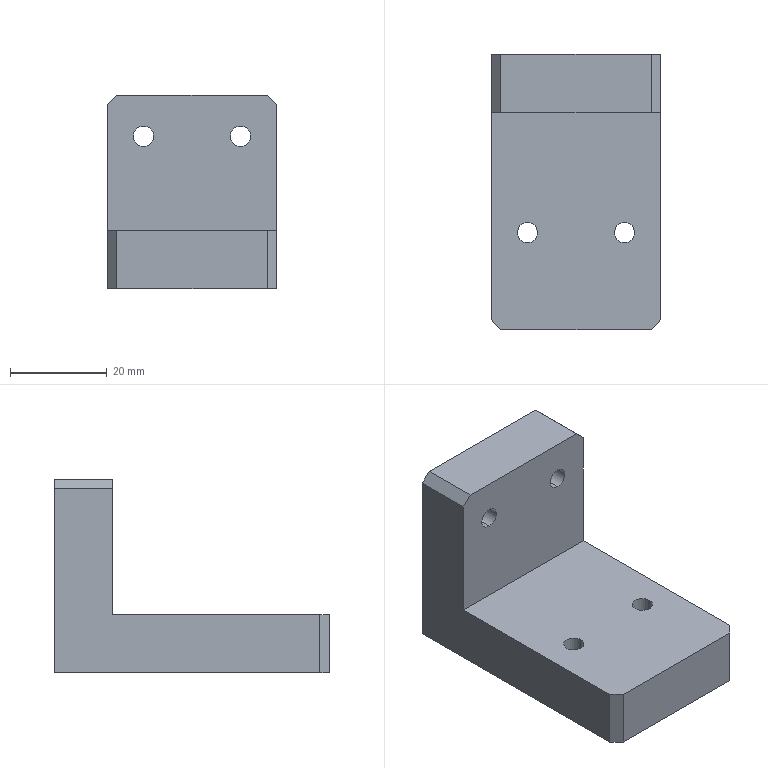Part | SolidWorks | features Chamfer 2, HoleWzd 2, Extrusion 1, ICE 1 | 1 solid | 28 faces | box 35 x 56.7 x 40 mm | volume 34458 mm3 | cylinder 12 | plane 12 | cone 4 | commonest cylinder face diameters 4.2 x12
STEP:
#1=CARTESIAN_POINT('',(-10.,15.95,4.4));
#2=VERTEX_POINT('',#1);
#3=CARTESIAN_POINT('',(-10.,15.95,8.6));
#4=VERTEX_POINT('',#3);
#5=CARTESIAN_POINT('',(-10.,15.95,6.5));
#6=DIRECTION('',(0.,1.,0.));
#7=DIRECTION('',(0.,0.,1.));
#8=AXIS2_PLACEMENT_3D('',#5,#6,#7);
#9=CIRCLE('',#8,2.1);
#10=EDGE_CURVE('',#2,#4,#9,.T.);
#11=ORIENTED_EDGE('',*,*,#10,.F.);
#12=CARTESIAN_POINT('',(-10.,28.35,4.4));
#13=VERTEX_POINT('',#12);
#14=CARTESIAN_POINT('',(-10.,28.35,4.4));
#15=DIRECTION('',(0.,1.,0.));
#16=VECTOR('',#15,1000.);
#17=LINE('',#14,#16);
#18=EDGE_CURVE('',#2,#13,#17,.T.);
#19=ORIENTED_EDGE('',*,*,#18,.T.);
#20=CARTESIAN_POINT('',(-10.,28.35,8.6));
#21=VERTEX_POINT('',#20);
#22=CARTESIAN_POINT('',(-10.,28.35,6.5));
#23=DIRECTION('',(0.,1.,0.));
#24=DIRECTION('',(0.,0.,1.));
#25=AXIS2_PLACEMENT_3D('',#22,#23,#24);
#26=CIRCLE('',#25,2.1);
#27=EDGE_CURVE('',#13,#21,#26,.T.);
#28=ORIENTED_EDGE('',*,*,#27,.T.);
#29=CARTESIAN_POINT('',(-10.,28.35,8.6));
#30=DIRECTION('',(0.,1.,0.));
#31=VECTOR('',#30,1000.);
#32=LINE('',#29,#31);
#33=EDGE_CURVE('',#4,#21,#32,.T.);
#34=ORIENTED_EDGE('',*,*,#33,.F.);
#35=EDGE_LOOP('',(#11,#19,#28,#34));
#36=FACE_OUTER_BOUND('',#35,.T.);
#37=CARTESIAN_POINT('',(-10.,28.35,6.5));
#38=DIRECTION('',(0.,1.,0.));
#39=DIRECTION('',(0.,0.,1.));
#40=AXIS2_PLACEMENT_3D('',#37,#38,#39);
#41=CYLINDRICAL_SURFACE('',#40,2.1);
#42=ADVANCED_FACE('',(#36),#41,.F.);
#43=CARTESIAN_POINT('',(-10.,14.688,6.5));
#44=VERTEX_POINT('',#43);
#45=CARTESIAN_POINT('',(-10.,15.95,8.6));
#46=DIRECTION('',(0.,0.515,0.8572));
#47=VECTOR('',#46,1000.);
#48=LINE('',#45,#47);
#49=EDGE_CURVE('',#44,#4,#48,.T.);
#50=ORIENTED_EDGE('',*,*,#49,.F.);
#51=CARTESIAN_POINT('',(-10.,15.95,4.4));
#52=DIRECTION('',(0.,0.515,-0.8572));
#53=VECTOR('',#52,1000.);
#54=LINE('',#51,#53);
#55=EDGE_CURVE('',#44,#2,#54,.T.);
#56=ORIENTED_EDGE('',*,*,#55,.T.);
#57=ORIENTED_EDGE('',*,*,#10,.T.);
#58=EDGE_LOOP('',(#50,#56,#57));
#59=FACE_OUTER_BOUND('',#58,.T.);
#60=CARTESIAN_POINT('',(-10.,15.95,6.5));
#61=DIRECTION('',(0.,1.,0.));
#62=DIRECTION('',(0.,0.,1.));
#63=AXIS2_PLACEMENT_3D('',#60,#61,#62);
#64=CONICAL_SURFACE('',#63,2.1,1.03);
#65=ADVANCED_FACE('',(#59),#64,.F.);
#66=CARTESIAN_POINT('',(10.,15.95,4.4));
#67=VERTEX_POINT('',#66);
#68=CARTESIAN_POINT('',(10.,15.95,8.6));
#69=VERTEX_POINT('',#68);
#70=CARTESIAN_POINT('',(10.,15.95,6.5));
#71=DIRECTION('',(0.,1.,0.));
#72=DIRECTION('',(0.,0.,1.));
#73=AXIS2_PLACEMENT_3D('',#70,#71,#72);
#74=CIRCLE('',#73,2.1);
#75=EDGE_CURVE('',#67,#69,#74,.T.);
#76=ORIENTED_EDGE('',*,*,#75,.F.);
#77=CARTESIAN_POINT('',(10.,28.35,4.4));
#78=VERTEX_POINT('',#77);
#79=CARTESIAN_POINT('',(10.,28.35,4.4));
#80=DIRECTION('',(0.,1.,0.));
#81=VECTOR('',#80,1000.);
#82=LINE('',#79,#81);
#83=EDGE_CURVE('',#67,#78,#82,.T.);
#84=ORIENTED_EDGE('',*,*,#83,.T.);
#85=CARTESIAN_POINT('',(10.,28.35,8.6));
#86=VERTEX_POINT('',#85);
#87=CARTESIAN_POINT('',(10.,28.35,6.5));
#88=DIRECTION('',(0.,1.,0.));
#89=DIRECTION('',(0.,0.,1.));
#90=AXIS2_PLACEMENT_3D('',#87,#88,#89);
#91=CIRCLE('',#90,2.1);
#92=EDGE_CURVE('',#78,#86,#91,.T.);
#93=ORIENTED_EDGE('',*,*,#92,.T.);
#94=CARTESIAN_POINT('',(10.,28.35,8.6));
#95=DIRECTION('',(0.,1.,0.));
#96=VECTOR('',#95,1000.);
#97=LINE('',#94,#96);
#98=EDGE_CURVE('',#69,#86,#97,.T.);
#99=ORIENTED_EDGE('',*,*,#98,.F.);
#100=EDGE_LOOP('',(#76,#84,#93,#99));
#101=FACE_OUTER_BOUND('',#100,.T.);
#102=CARTESIAN_POINT('',(10.,28.35,6.5));
#103=DIRECTION('',(0.,1.,0.));
#104=DIRECTION('',(0.,0.,1.));
#105=AXIS2_PLACEMENT_3D('',#102,#103,#104);
#106=CYLINDRICAL_SURFACE('',#105,2.1);
#107=ADVANCED_FACE('',(#101),#106,.F.);
#108=CARTESIAN_POINT('',(10.,14.688,6.5));
#109=VERTEX_POINT('',#108);
#110=CARTESIAN_POINT('',(10.,15.95,8.6));
#111=DIRECTION('',(0.,0.515,0.8572));
#112=VECTOR('',#111,1000.);
#113=LINE('',#110,#112);
#114=EDGE_CURVE('',#109,#69,#113,.T.);
#115=ORIENTED_EDGE('',*,*,#114,.F.);
#116=CARTESIAN_POINT('',(10.,15.95,4.4));
#117=DIRECTION('',(0.,0.515,-0.8572));
#118=VECTOR('',#117,1000.);
#119=LINE('',#116,#118);
#120=EDGE_CURVE('',#109,#67,#119,.T.);
#121=ORIENTED_EDGE('',*,*,#120,.T.);
#122=ORIENTED_EDGE('',*,*,#75,.T.);
#123=EDGE_LOOP('',(#115,#121,#122));
#124=FACE_OUTER_BOUND('',#123,.T.);
#125=CARTESIAN_POINT('',(10.,15.95,6.5));
#126=DIRECTION('',(0.,1.,0.));
#127=DIRECTION('',(0.,0.,1.));
#128=AXIS2_PLACEMENT_3D('',#125,#126,#127);
#129=CONICAL_SURFACE('',#128,2.1,1.03);
#130=ADVANCED_FACE('',(#124),#129,.F.);
#131=CARTESIAN_POINT('',(-10.,16.35,33.6));
#132=VERTEX_POINT('',#131);
#133=CARTESIAN_POINT('',(-10.,16.35,29.4));
#134=VERTEX_POINT('',#133);
#135=CARTESIAN_POINT('',(-10.,16.35,31.5));
#136=DIRECTION('',(0.,-1.,0.));
#137=DIRECTION('',(0.,0.,-1.));
#138=AXIS2_PLACEMENT_3D('',#135,#136,#137);
#139=CIRCLE('',#138,2.1);
#140=EDGE_CURVE('',#132,#134,#139,.T.);
#141=ORIENTED_EDGE('',*,*,#140,.T.);
#142=CARTESIAN_POINT('',(-10.,28.35,29.4));
#143=VERTEX_POINT('',#142);
#144=CARTESIAN_POINT('',(-10.,28.35,29.4));
#145=DIRECTION('',(0.,1.,0.));
#146=VECTOR('',#145,1000.);
#147=LINE('',#144,#146);
#148=EDGE_CURVE('',#134,#143,#147,.T.);
#149=ORIENTED_EDGE('',*,*,#148,.T.);
#150=CARTESIAN_POINT('',(-10.,28.35,33.6));
#151=VERTEX_POINT('',#150);
#152=CARTESIAN_POINT('',(-10.,28.35,31.5));
#153=DIRECTION('',(0.,1.,0.));
#154=DIRECTION('',(0.,0.,1.));
#155=AXIS2_PLACEMENT_3D('',#152,#153,#154);
#156=CIRCLE('',#155,2.1);
#157=EDGE_CURVE('',#143,#151,#156,.T.);
#158=ORIENTED_EDGE('',*,*,#157,.T.);
#159=CARTESIAN_POINT('',(-10.,28.35,33.6));
#160=DIRECTION('',(0.,1.,0.));
#161=VECTOR('',#160,1000.);
#162=LINE('',#159,#161);
#163=EDGE_CURVE('',#132,#151,#162,.T.);
#164=ORIENTED_EDGE('',*,*,#163,.F.);
#165=EDGE_LOOP('',(#141,#149,#158,#164));
#166=FACE_OUTER_BOUND('',#165,.T.);
#167=CARTESIAN_POINT('',(-10.,28.35,31.5));
#168=DIRECTION('',(0.,1.,0.));
#169=DIRECTION('',(0.,0.,1.));
#170=AXIS2_PLACEMENT_3D('',#167,#168,#169);
#171=CYLINDRICAL_SURFACE('',#170,2.1);
#172=ADVANCED_FACE('',(#166),#171,.F.);
#173=CARTESIAN_POINT('',(10.,16.35,33.6));
#174=VERTEX_POINT('',#173);
#175=CARTESIAN_POINT('',(10.,16.35,29.4));
#176=VERTEX_POINT('',#175);
#177=CARTESIAN_POINT('',(10.,16.35,31.5));
#178=DIRECTION('',(0.,-1.,0.));
#179=DIRECTION('',(0.,0.,-1.));
#180=AXIS2_PLACEMENT_3D('',#177,#178,#179);
#181=CIRCLE('',#180,2.1);
#182=EDGE_CURVE('',#174,#176,#181,.T.);
#183=ORIENTED_EDGE('',*,*,#182,.T.);
#184=CARTESIAN_POINT('',(10.,28.35,29.4));
#185=VERTEX_POINT('',#184);
#186=CARTESIAN_POINT('',(10.,28.35,29.4));
#187=DIRECTION('',(0.,1.,0.));
#188=VECTOR('',#187,1000.);
#189=LINE('',#186,#188);
#190=EDGE_CURVE('',#176,#185,#189,.T.);
#191=ORIENTED_EDGE('',*,*,#190,.T.);
#192=CARTESIAN_POINT('',(10.,28.35,33.6));
#193=VERTEX_POINT('',#192);
#194=CARTESIAN_POINT('',(10.,28.35,31.5));
#195=DIRECTION('',(0.,1.,0.));
#196=DIRECTION('',(0.,0.,1.));
#197=AXIS2_PLACEMENT_3D('',#194,#195,#196);
#198=CIRCLE('',#197,2.1);
#199=EDGE_CURVE('',#185,#193,#198,.T.);
#200=ORIENTED_EDGE('',*,*,#199,.T.);
#201=CARTESIAN_POINT('',(10.,28.35,33.6));
#202=DIRECTION('',(0.,1.,0.));
#203=VECTOR('',#202,1000.);
#204=LINE('',#201,#203);
#205=EDGE_CURVE('',#174,#193,#204,.T.);
#206=ORIENTED_EDGE('',*,*,#205,.F.);
#207=EDGE_LOOP('',(#183,#191,#200,#206));
#208=FACE_OUTER_BOUND('',#207,.T.);
#209=CARTESIAN_POINT('',(10.,28.35,31.5));
#210=DIRECTION('',(0.,1.,0.));
#211=DIRECTION('',(0.,0.,1.));
#212=AXIS2_PLACEMENT_3D('',#209,#210,#211);
#213=CYLINDRICAL_SURFACE('',#212,2.1);
#214=ADVANCED_FACE('',(#208),#213,.F.);
#215=CARTESIAN_POINT('',(12.1,-8.35,12.));
#216=VERTEX_POINT('',#215);
#217=CARTESIAN_POINT('',(7.9,-8.35,12.));
#218=VERTEX_POINT('',#217);
#219=CARTESIAN_POINT('',(10.,-8.35,12.));
#220=DIRECTION('',(0.,0.,-1.));
#221=DIRECTION('',(-1.,0.,0.));
#222=AXIS2_PLACEMENT_3D('',#219,#220,#221);
#223=CIRCLE('',#222,2.1);
#224=EDGE_CURVE('',#216,#218,#223,.T.);
#225=ORIENTED_EDGE('',*,*,#224,.F.);
#226=CARTESIAN_POINT('',(12.1,-8.35,0.));
#227=VERTEX_POINT('',#226);
#228=CARTESIAN_POINT('',(12.1,-8.35,0.));
#229=DIRECTION('',(0.,0.,-1.));
#230=VECTOR('',#229,1000.);
#231=LINE('',#228,#230);
#232=EDGE_CURVE('',#216,#227,#231,.T.);
#233=ORIENTED_EDGE('',*,*,#232,.T.);
#234=CARTESIAN_POINT('',(7.9,-8.35,0.));
#235=VERTEX_POINT('',#234);
#236=CARTESIAN_POINT('',(10.,-8.35,0.));
#237=DIRECTION('',(0.,0.,-1.));
#238=DIRECTION('',(-1.,0.,0.));
#239=AXIS2_PLACEMENT_3D('',#236,#237,#238);
#240=CIRCLE('',#239,2.1);
#241=EDGE_CURVE('',#227,#235,#240,.T.);
#242=ORIENTED_EDGE('',*,*,#241,.T.);
#243=CARTESIAN_POINT('',(7.9,-8.35,0.));
#244=DIRECTION('',(0.,0.,-1.));
#245=VECTOR('',#244,1000.);
#246=LINE('',#243,#245);
#247=EDGE_CURVE('',#218,#235,#246,.T.);
#248=ORIENTED_EDGE('',*,*,#247,.F.);
#249=EDGE_LOOP('',(#225,#233,#242,#248));
#250=FACE_OUTER_BOUND('',#249,.T.);
#251=CARTESIAN_POINT('',(10.,-8.35,0.));
#252=DIRECTION('',(0.,0.,-1.));
#253=DIRECTION('',(-1.,0.,0.));
#254=AXIS2_PLACEMENT_3D('',#251,#252,#253);
#255=CYLINDRICAL_SURFACE('',#254,2.1);
#256=ADVANCED_FACE('',(#250),#255,.F.);
#257=CARTESIAN_POINT('',(-7.9,-8.35,12.));
#258=VERTEX_POINT('',#257);
#259=CARTESIAN_POINT('',(-12.1,-8.35,12.));
#260=VERTEX_POINT('',#259);
#261=CARTESIAN_POINT('',(-10.,-8.35,12.));
#262=DIRECTION('',(0.,0.,-1.));
#263=DIRECTION('',(-1.,0.,0.));
#264=AXIS2_PLACEMENT_3D('',#261,#262,#263);
#265=CIRCLE('',#264,2.1);
#266=EDGE_CURVE('',#258,#260,#265,.T.);
#267=ORIENTED_EDGE('',*,*,#266,.F.);
#268=CARTESIAN_POINT('',(-7.9,-8.35,0.));
#269=VERTEX_POINT('',#268);
#270=CARTESIAN_POINT('',(-7.9,-8.35,0.));
#271=DIRECTION('',(0.,0.,-1.));
#272=VECTOR('',#271,1000.);
#273=LINE('',#270,#272);
#274=EDGE_CURVE('',#258,#269,#273,.T.);
#275=ORIENTED_EDGE('',*,*,#274,.T.);
#276=CARTESIAN_POINT('',(-12.1,-8.35,0.));
#277=VERTEX_POINT('',#276);
#278=CARTESIAN_POINT('',(-10.,-8.35,0.));
#279=DIRECTION('',(0.,0.,-1.));
#280=DIRECTION('',(-1.,0.,0.));
#281=AXIS2_PLACEMENT_3D('',#278,#279,#280);
#282=CIRCLE('',#281,2.1);
#283=EDGE_CURVE('',#269,#277,#282,.T.);
#284=ORIENTED_EDGE('',*,*,#283,.T.);
#285=CARTESIAN_POINT('',(-12.1,-8.35,0.));
#286=DIRECTION('',(0.,0.,-1.));
#287=VECTOR('',#286,1000.);
#288=LINE('',#285,#287);
#289=EDGE_CURVE('',#260,#277,#288,.T.);
#290=ORIENTED_EDGE('',*,*,#289,.F.);
#291=EDGE_LOOP('',(#267,#275,#284,#290));
#292=FACE_OUTER_BOUND('',#291,.T.);
#293=CARTESIAN_POINT('',(-10.,-8.35,0.));
#294=DIRECTION('',(0.,0.,-1.));
#295=DIRECTION('',(-1.,0.,0.));
#296=AXIS2_PLACEMENT_3D('',#293,#294,#295);
#297=CYLINDRICAL_SURFACE('',#296,2.1);
#298=ADVANCED_FACE('',(#292),#297,.F.);
#299=CARTESIAN_POINT('',(-17.5,16.35,12.));
#300=VERTEX_POINT('',#299);
#301=CARTESIAN_POINT('',(-17.5,16.35,38.));
#302=VERTEX_POINT('',#301);
#303=CARTESIAN_POINT('',(-17.5,16.35,12.));
#304=DIRECTION('',(0.,0.,1.));
#305=VECTOR('',#304,1000.);
#306=LINE('',#303,#305);
#307=EDGE_CURVE('',#300,#302,#306,.T.);
#308=ORIENTED_EDGE('',*,*,#307,.T.);
#309=CARTESIAN_POINT('',(-17.5,28.35,38.));
#310=VERTEX_POINT('',#309);
#311=CARTESIAN_POINT('',(-17.5,-28.35,38.));
#312=DIRECTION('',(0.,1.,0.));
#313=VECTOR('',#312,1000.);
#314=LINE('',#311,#313);
#315=EDGE_CURVE('',#302,#310,#314,.T.);
#316=ORIENTED_EDGE('',*,*,#315,.T.);
#317=CARTESIAN_POINT('',(-17.5,28.35,0.));
#318=VERTEX_POINT('',#317);
#319=CARTESIAN_POINT('',(-17.5,28.35,12.));
#320=DIRECTION('',(0.,0.,-1.));
#321=VECTOR('',#320,1000.);
#322=LINE('',#319,#321);
#323=EDGE_CURVE('',#310,#318,#322,.T.);
#324=ORIENTED_EDGE('',*,*,#323,.T.);
#325=CARTESIAN_POINT('',(-17.5,-26.35,0.));
#326=VERTEX_POINT('',#325);
#327=CARTESIAN_POINT('',(-17.5,-28.35,0.));
#328=DIRECTION('',(0.,1.,0.));
#329=VECTOR('',#328,1000.);
#330=LINE('',#327,#329);
#331=EDGE_CURVE('',#326,#318,#330,.T.);
#332=ORIENTED_EDGE('',*,*,#331,.F.);
#333=CARTESIAN_POINT('',(-17.5,-26.35,12.));
#334=VERTEX_POINT('',#333);
#335=CARTESIAN_POINT('',(-17.5,-26.35,12.));
#336=DIRECTION('',(0.,0.,1.));
#337=VECTOR('',#336,1000.);
#338=LINE('',#335,#337);
#339=EDGE_CURVE('',#326,#334,#338,.T.);
#340=ORIENTED_EDGE('',*,*,#339,.T.);
#341=CARTESIAN_POINT('',(-17.5,-28.35,12.));
#342=DIRECTION('',(0.,1.,0.));
#343=VECTOR('',#342,1000.);
#344=LINE('',#341,#343);
#345=EDGE_CURVE('',#334,#300,#344,.T.);
#346=ORIENTED_EDGE('',*,*,#345,.T.);
#347=EDGE_LOOP('',(#308,#316,#324,#332,#340,#346));
#348=FACE_OUTER_BOUND('',#347,.T.);
#349=CARTESIAN_POINT('',(-17.5,-28.35,12.));
#350=DIRECTION('',(-1.,0.,0.));
#351=DIRECTION('',(0.,0.,1.));
#352=AXIS2_PLACEMENT_3D('',#349,#350,#351);
#353=PLANE('',#352);
#354=ADVANCED_FACE('',(#348),#353,.T.);
#355=CARTESIAN_POINT('',(-15.5,-28.35,0.));
#356=VERTEX_POINT('',#355);
#357=CARTESIAN_POINT('',(15.5,-28.35,0.));
#358=VERTEX_POINT('',#357);
#359=CARTESIAN_POINT('',(-17.5,-28.35,0.));
#360=DIRECTION('',(1.,0.,0.));
#361=VECTOR('',#360,1000.);
#362=LINE('',#359,#361);
#363=EDGE_CURVE('',#356,#358,#362,.T.);
#364=ORIENTED_EDGE('',*,*,#363,.T.);
#365=CARTESIAN_POINT('',(15.5,-28.35,12.));
#366=VERTEX_POINT('',#365);
#367=CARTESIAN_POINT('',(15.5,-28.35,12.));
#368=DIRECTION('',(0.,0.,1.));
#369=VECTOR('',#368,1000.);
#370=LINE('',#367,#369);
#371=EDGE_CURVE('',#358,#366,#370,.T.);
#372=ORIENTED_EDGE('',*,*,#371,.T.);
#373=CARTESIAN_POINT('',(-15.5,-28.35,12.));
#374=VERTEX_POINT('',#373);
#375=CARTESIAN_POINT('',(-17.5,-28.35,12.));
#376=DIRECTION('',(1.,0.,0.));
#377=VECTOR('',#376,1000.);
#378=LINE('',#375,#377);
#379=EDGE_CURVE('',#374,#366,#378,.T.);
#380=ORIENTED_EDGE('',*,*,#379,.F.);
#381=CARTESIAN_POINT('',(-15.5,-28.35,0.));
#382=DIRECTION('',(0.,0.,-1.));
#383=VECTOR('',#382,1000.);
#384=LINE('',#381,#383);
#385=EDGE_CURVE('',#374,#356,#384,.T.);
#386=ORIENTED_EDGE('',*,*,#385,.T.);
#387=EDGE_LOOP('',(#364,#372,#380,#386));
#388=FACE_OUTER_BOUND('',#387,.T.);
#389=CARTESIAN_POINT('',(-17.5,-28.35,12.));
#390=DIRECTION('',(0.,1.,0.));
#391=DIRECTION('',(0.,0.,1.));
#392=AXIS2_PLACEMENT_3D('',#389,#390,#391);
#393=PLANE('',#392);
#394=ADVANCED_FACE('',(#388),#393,.F.);
#395=CARTESIAN_POINT('',(17.5,28.35,38.));
#396=VERTEX_POINT('',#395);
#397=CARTESIAN_POINT('',(17.5,28.35,0.));
#398=VERTEX_POINT('',#397);
#399=CARTESIAN_POINT('',(17.5,28.35,12.));
#400=DIRECTION('',(0.,0.,-1.));
#401=VECTOR('',#400,1000.);
#402=LINE('',#399,#401);
#403=EDGE_CURVE('',#396,#398,#402,.T.);
#404=ORIENTED_EDGE('',*,*,#403,.F.);
#405=CARTESIAN_POINT('',(17.5,16.35,38.));
#406=VERTEX_POINT('',#405);
#407=CARTESIAN_POINT('',(17.5,16.35,38.));
#408=DIRECTION('',(0.,-1.,0.));
#409=VECTOR('',#408,1000.);
#410=LINE('',#407,#409);
#411=EDGE_CURVE('',#396,#406,#410,.T.);
#412=ORIENTED_EDGE('',*,*,#411,.T.);
#413=CARTESIAN_POINT('',(17.5,16.35,12.));
#414=VERTEX_POINT('',#413);
#415=CARTESIAN_POINT('',(17.5,16.35,12.));
#416=DIRECTION('',(0.,0.,-1.));
#417=VECTOR('',#416,1000.);
#418=LINE('',#415,#417);
#419=EDGE_CURVE('',#406,#414,#418,.T.);
#420=ORIENTED_EDGE('',*,*,#419,.T.);
#421=CARTESIAN_POINT('',(17.5,-26.35,12.));
#422=VERTEX_POINT('',#421);
#423=CARTESIAN_POINT('',(17.5,-28.35,12.));
#424=DIRECTION('',(0.,1.,0.));
#425=VECTOR('',#424,1000.);
#426=LINE('',#423,#425);
#427=EDGE_CURVE('',#422,#414,#426,.T.);
#428=ORIENTED_EDGE('',*,*,#427,.F.);
#429=CARTESIAN_POINT('',(17.5,-26.35,0.));
#430=VERTEX_POINT('',#429);
#431=CARTESIAN_POINT('',(17.5,-26.35,12.));
#432=DIRECTION('',(0.,0.,-1.));
#433=VECTOR('',#432,1000.);
#434=LINE('',#431,#433);
#435=EDGE_CURVE('',#422,#430,#434,.T.);
#436=ORIENTED_EDGE('',*,*,#435,.T.);
#437=CARTESIAN_POINT('',(17.5,-28.35,0.));
#438=DIRECTION('',(0.,1.,0.));
#439=VECTOR('',#438,1000.);
#440=LINE('',#437,#439);
#441=EDGE_CURVE('',#430,#398,#440,.T.);
#442=ORIENTED_EDGE('',*,*,#441,.T.);
#443=EDGE_LOOP('',(#404,#412,#420,#428,#436,#442));
#444=FACE_OUTER_BOUND('',#443,.T.);
#445=CARTESIAN_POINT('',(17.5,-28.35,12.));
#446=DIRECTION('',(-1.,0.,0.));
#447=DIRECTION('',(0.,0.,1.));
#448=AXIS2_PLACEMENT_3D('',#445,#446,#447);
#449=PLANE('',#448);
#450=ADVANCED_FACE('',(#444),#449,.F.);
#451=CARTESIAN_POINT('',(-10.,28.35,6.5));
#452=DIRECTION('',(0.,1.,0.));
#453=DIRECTION('',(0.,0.,1.));
#454=AXIS2_PLACEMENT_3D('',#451,#452,#453);
#455=CIRCLE('',#454,2.1);
#456=EDGE_CURVE('',#21,#13,#455,.T.);
#457=ORIENTED_EDGE('',*,*,#456,.F.);
#458=ORIENTED_EDGE('',*,*,#27,.F.);
#459=EDGE_LOOP('',(#457,#458));
#460=FACE_BOUND('',#459,.T.);
#461=CARTESIAN_POINT('',(10.,28.35,6.5));
#462=DIRECTION('',(0.,1.,0.));
#463=DIRECTION('',(0.,0.,1.));
#464=AXIS2_PLACEMENT_3D('',#461,#462,#463);
#465=CIRCLE('',#464,2.1);
#466=EDGE_CURVE('',#86,#78,#465,.T.);
#467=ORIENTED_EDGE('',*,*,#466,.F.);
#468=ORIENTED_EDGE('',*,*,#92,.F.);
#469=EDGE_LOOP('',(#467,#468));
#470=FACE_BOUND('',#469,.T.);
#471=CARTESIAN_POINT('',(-10.,28.35,31.5));
#472=DIRECTION('',(0.,1.,0.));
#473=DIRECTION('',(0.,0.,1.));
#474=AXIS2_PLACEMENT_3D('',#471,#472,#473);
#475=CIRCLE('',#474,2.1);
#476=EDGE_CURVE('',#151,#143,#475,.T.);
#477=ORIENTED_EDGE('',*,*,#476,.F.);
#478=ORIENTED_EDGE('',*,*,#157,.F.);
#479=EDGE_LOOP('',(#477,#478));
#480=FACE_BOUND('',#479,.T.);
#481=CARTESIAN_POINT('',(10.,28.35,31.5));
#482=DIRECTION('',(0.,1.,0.));
#483=DIRECTION('',(0.,0.,1.));
#484=AXIS2_PLACEMENT_3D('',#481,#482,#483);
#485=CIRCLE('',#484,2.1);
#486=EDGE_CURVE('',#193,#185,#485,.T.);
#487=ORIENTED_EDGE('',*,*,#486,.F.);
#488=ORIENTED_EDGE('',*,*,#199,.F.);
#489=EDGE_LOOP('',(#487,#488));
#490=FACE_BOUND('',#489,.T.);
#491=CARTESIAN_POINT('',(15.5,28.35,40.));
#492=VERTEX_POINT('',#491);
#493=CARTESIAN_POINT('',(-15.5,28.35,40.));
#494=VERTEX_POINT('',#493);
#495=CARTESIAN_POINT('',(47.963,28.35,40.));
#496=DIRECTION('',(-1.,0.,0.));
#497=VECTOR('',#496,1000.);
#498=LINE('',#495,#497);
#499=EDGE_CURVE('',#492,#494,#498,.T.);
#500=ORIENTED_EDGE('',*,*,#499,.F.);
#501=CARTESIAN_POINT('',(13.,28.35,42.5));
#502=DIRECTION('',(0.7071,0.,-0.7071));
#503=VECTOR('',#502,1000.);
#504=LINE('',#501,#503);
#505=EDGE_CURVE('',#492,#396,#504,.T.);
#506=ORIENTED_EDGE('',*,*,#505,.T.);
#507=ORIENTED_EDGE('',*,*,#403,.T.);
#508=CARTESIAN_POINT('',(-17.5,28.35,0.));
#509=DIRECTION('',(1.,0.,0.));
#510=VECTOR('',#509,1000.);
#511=LINE('',#508,#510);
#512=EDGE_CURVE('',#318,#398,#511,.T.);
#513=ORIENTED_EDGE('',*,*,#512,.F.);
#514=ORIENTED_EDGE('',*,*,#323,.F.);
#515=CARTESIAN_POINT('',(-30.5,28.35,25.));
#516=DIRECTION('',(0.7071,0.,0.7071));
#517=VECTOR('',#516,1000.);
#518=LINE('',#515,#517);
#519=EDGE_CURVE('',#310,#494,#518,.T.);
#520=ORIENTED_EDGE('',*,*,#519,.T.);
#521=EDGE_LOOP('',(#500,#506,#507,#513,#514,#520));
#522=FACE_OUTER_BOUND('',#521,.T.);
#523=CARTESIAN_POINT('',(-17.5,28.35,12.));
#524=DIRECTION('',(0.,1.,0.));
#525=DIRECTION('',(0.,0.,1.));
#526=AXIS2_PLACEMENT_3D('',#523,#524,#525);
#527=PLANE('',#526);
#528=ADVANCED_FACE('',(#460,#470,#480,#490,#522),#527,.T.);
#529=CARTESIAN_POINT('',(10.,-8.35,12.));
#530=DIRECTION('',(0.,0.,-1.));
#531=DIRECTION('',(-1.,0.,0.));
#532=AXIS2_PLACEMENT_3D('',#529,#530,#531);
#533=CIRCLE('',#532,2.1);
#534=EDGE_CURVE('',#218,#216,#533,.T.);
#535=ORIENTED_EDGE('',*,*,#534,.T.);
#536=ORIENTED_EDGE('',*,*,#224,.T.);
#537=EDGE_LOOP('',(#535,#536));
#538=FACE_BOUND('',#537,.T.);
#539=CARTESIAN_POINT('',(-10.,-8.35,12.));
#540=DIRECTION('',(0.,0.,-1.));
#541=DIRECTION('',(-1.,0.,0.));
#542=AXIS2_PLACEMENT_3D('',#539,#540,#541);
#543=CIRCLE('',#542,2.1);
#544=EDGE_CURVE('',#260,#258,#543,.T.);
#545=ORIENTED_EDGE('',*,*,#544,.T.);
#546=ORIENTED_EDGE('',*,*,#266,.T.);
#547=EDGE_LOOP('',(#545,#546));
#548=FACE_BOUND('',#547,.T.);
#549=ORIENTED_EDGE('',*,*,#427,.T.);
#550=CARTESIAN_POINT('',(47.963,16.35,12.));
#551=DIRECTION('',(-1.,0.,0.));
#552=VECTOR('',#551,1000.);
#553=LINE('',#550,#552);
#554=EDGE_CURVE('',#414,#300,#553,.T.);
#555=ORIENTED_EDGE('',*,*,#554,.T.);
#556=ORIENTED_EDGE('',*,*,#345,.F.);
#557=CARTESIAN_POINT('',(-15.5,-28.35,12.));
#558=DIRECTION('',(0.7071,-0.7071,0.));
#559=VECTOR('',#558,1000.);
#560=LINE('',#557,#559);
#561=EDGE_CURVE('',#334,#374,#560,.T.);
#562=ORIENTED_EDGE('',*,*,#561,.T.);
#563=ORIENTED_EDGE('',*,*,#379,.T.);
#564=CARTESIAN_POINT('',(17.5,-26.35,12.));
#565=DIRECTION('',(0.7071,0.7071,0.));
#566=VECTOR('',#565,1000.);
#567=LINE('',#564,#566);
#568=EDGE_CURVE('',#366,#422,#567,.T.);
#569=ORIENTED_EDGE('',*,*,#568,.T.);
#570=EDGE_LOOP('',(#549,#555,#556,#562,#563,#569));
#571=FACE_OUTER_BOUND('',#570,.T.);
#572=CARTESIAN_POINT('',(0.,0.,12.));
#573=DIRECTION('',(0.,0.,-1.));
#574=DIRECTION('',(-1.,0.,0.));
#575=AXIS2_PLACEMENT_3D('',#572,#573,#574);
#576=PLANE('',#575);
#577=ADVANCED_FACE('',(#538,#548,#571),#576,.F.);
#578=CARTESIAN_POINT('',(10.,-8.35,0.));
#579=DIRECTION('',(0.,0.,-1.));
#580=DIRECTION('',(-1.,0.,0.));
#581=AXIS2_PLACEMENT_3D('',#578,#579,#580);
#582=CIRCLE('',#581,2.1);
#583=EDGE_CURVE('',#235,#227,#582,.T.);
#584=ORIENTED_EDGE('',*,*,#583,.F.);
#585=ORIENTED_EDGE('',*,*,#241,.F.);
#586=EDGE_LOOP('',(#584,#585));
#587=FACE_BOUND('',#586,.T.);
#588=CARTESIAN_POINT('',(-10.,-8.35,0.));
#589=DIRECTION('',(0.,0.,-1.));
#590=DIRECTION('',(-1.,0.,0.));
#591=AXIS2_PLACEMENT_3D('',#588,#589,#590);
#592=CIRCLE('',#591,2.1);
#593=EDGE_CURVE('',#277,#269,#592,.T.);
#594=ORIENTED_EDGE('',*,*,#593,.F.);
#595=ORIENTED_EDGE('',*,*,#283,.F.);
#596=EDGE_LOOP('',(#594,#595));
#597=FACE_BOUND('',#596,.T.);
#598=ORIENTED_EDGE('',*,*,#441,.F.);
#599=CARTESIAN_POINT('',(21.925,-21.925,0.));
#600=DIRECTION('',(-0.7071,-0.7071,0.));
#601=VECTOR('',#600,1000.);
#602=LINE('',#599,#601);
#603=EDGE_CURVE('',#430,#358,#602,.T.);
#604=ORIENTED_EDGE('',*,*,#603,.T.);
#605=ORIENTED_EDGE('',*,*,#363,.F.);
#606=CARTESIAN_POINT('',(-21.925,-21.925,0.));
#607=DIRECTION('',(-0.7071,0.7071,0.));
#608=VECTOR('',#607,1000.);
#609=LINE('',#606,#608);
#610=EDGE_CURVE('',#356,#326,#609,.T.);
#611=ORIENTED_EDGE('',*,*,#610,.T.);
#612=ORIENTED_EDGE('',*,*,#331,.T.);
#613=ORIENTED_EDGE('',*,*,#512,.T.);
#614=EDGE_LOOP('',(#598,#604,#605,#611,#612,#613));
#615=FACE_OUTER_BOUND('',#614,.T.);
#616=CARTESIAN_POINT('',(0.,0.,0.));
#617=DIRECTION('',(0.,0.,-1.));
#618=DIRECTION('',(-1.,0.,0.));
#619=AXIS2_PLACEMENT_3D('',#616,#617,#618);
#620=PLANE('',#619);
#621=ADVANCED_FACE('',(#587,#597,#615),#620,.T.);
#622=ORIENTED_EDGE('',*,*,#568,.F.);
#623=ORIENTED_EDGE('',*,*,#371,.F.);
#624=ORIENTED_EDGE('',*,*,#603,.F.);
#625=ORIENTED_EDGE('',*,*,#435,.F.);
#626=EDGE_LOOP('',(#622,#623,#624,#625));
#627=FACE_OUTER_BOUND('',#626,.T.);
#628=CARTESIAN_POINT('',(17.5,-26.35,12.));
#629=DIRECTION('',(-0.7071,0.7071,0.));
#630=DIRECTION('',(0.,0.,-1.));
#631=AXIS2_PLACEMENT_3D('',#628,#629,#630);
#632=PLANE('',#631);
#633=ADVANCED_FACE('',(#627),#632,.F.);
#634=ORIENTED_EDGE('',*,*,#561,.F.);
#635=ORIENTED_EDGE('',*,*,#339,.F.);
#636=ORIENTED_EDGE('',*,*,#610,.F.);
#637=ORIENTED_EDGE('',*,*,#385,.F.);
#638=EDGE_LOOP('',(#634,#635,#636,#637));
#639=FACE_OUTER_BOUND('',#638,.T.);
#640=CARTESIAN_POINT('',(-15.5,-28.35,12.));
#641=DIRECTION('',(-0.7071,-0.7071,0.));
#642=DIRECTION('',(0.,0.,1.));
#643=AXIS2_PLACEMENT_3D('',#640,#641,#642);
#644=PLANE('',#643);
#645=ADVANCED_FACE('',(#639),#644,.T.);
#646=CARTESIAN_POINT('',(15.5,16.35,40.));
#647=VERTEX_POINT('',#646);
#648=CARTESIAN_POINT('',(-15.5,16.35,40.));
#649=VERTEX_POINT('',#648);
#650=CARTESIAN_POINT('',(47.963,16.35,40.));
#651=DIRECTION('',(-1.,0.,0.));
#652=VECTOR('',#651,1000.);
#653=LINE('',#650,#652);
#654=EDGE_CURVE('',#647,#649,#653,.T.);
#655=ORIENTED_EDGE('',*,*,#654,.F.);
#656=CARTESIAN_POINT('',(15.5,28.35,40.));
#657=DIRECTION('',(0.,1.,0.));
#658=VECTOR('',#657,1000.);
#659=LINE('',#656,#658);
#660=EDGE_CURVE('',#647,#492,#659,.T.);
#661=ORIENTED_EDGE('',*,*,#660,.T.);
#662=ORIENTED_EDGE('',*,*,#499,.T.);
#663=CARTESIAN_POINT('',(-15.5,28.35,40.));
#664=DIRECTION('',(0.,-1.,0.));
#665=VECTOR('',#664,1000.);
#666=LINE('',#663,#665);
#667=EDGE_CURVE('',#494,#649,#666,.T.);
#668=ORIENTED_EDGE('',*,*,#667,.T.);
#669=EDGE_LOOP('',(#655,#661,#662,#668));
#670=FACE_OUTER_BOUND('',#669,.T.);
#671=CARTESIAN_POINT('',(47.963,28.35,40.));
#672=DIRECTION('',(0.,0.,1.));
#673=DIRECTION('',(1.,0.,0.));
#674=AXIS2_PLACEMENT_3D('',#671,#672,#673);
#675=PLANE('',#674);
#676=ADVANCED_FACE('',(#670),#675,.T.);
#677=ORIENTED_EDGE('',*,*,#140,.F.);
#678=CARTESIAN_POINT('',(-10.,16.35,31.5));
#679=DIRECTION('',(0.,-1.,0.));
#680=DIRECTION('',(0.,0.,-1.));
#681=AXIS2_PLACEMENT_3D('',#678,#679,#680);
#682=CIRCLE('',#681,2.1);
#683=EDGE_CURVE('',#134,#132,#682,.T.);
#684=ORIENTED_EDGE('',*,*,#683,.F.);
#685=EDGE_LOOP('',(#677,#684));
#686=FACE_BOUND('',#685,.T.);
#687=ORIENTED_EDGE('',*,*,#182,.F.);
#688=CARTESIAN_POINT('',(10.,16.35,31.5));
#689=DIRECTION('',(0.,-1.,0.));
#690=DIRECTION('',(0.,0.,-1.));
#691=AXIS2_PLACEMENT_3D('',#688,#689,#690);
#692=CIRCLE('',#691,2.1);
#693=EDGE_CURVE('',#176,#174,#692,.T.);
#694=ORIENTED_EDGE('',*,*,#693,.F.);
#695=EDGE_LOOP('',(#687,#694));
#696=FACE_BOUND('',#695,.T.);
#697=ORIENTED_EDGE('',*,*,#419,.F.);
#698=CARTESIAN_POINT('',(45.732,16.35,9.768));
#699=DIRECTION('',(-0.7071,0.,0.7071));
#700=VECTOR('',#699,1000.);
#701=LINE('',#698,#700);
#702=EDGE_CURVE('',#406,#647,#701,.T.);
#703=ORIENTED_EDGE('',*,*,#702,.T.);
#704=ORIENTED_EDGE('',*,*,#654,.T.);
#705=CARTESIAN_POINT('',(2.232,16.35,57.732));
#706=DIRECTION('',(-0.7071,0.,-0.7071));
#707=VECTOR('',#706,1000.);
#708=LINE('',#705,#707);
#709=EDGE_CURVE('',#649,#302,#708,.T.);
#710=ORIENTED_EDGE('',*,*,#709,.T.);
#711=ORIENTED_EDGE('',*,*,#307,.F.);
#712=ORIENTED_EDGE('',*,*,#554,.F.);
#713=EDGE_LOOP('',(#697,#703,#704,#710,#711,#712));
#714=FACE_OUTER_BOUND('',#713,.T.);
#715=CARTESIAN_POINT('',(47.963,16.35,12.));
#716=DIRECTION('',(0.,-1.,0.));
#717=DIRECTION('',(0.,0.,-1.));
#718=AXIS2_PLACEMENT_3D('',#715,#716,#717);
#719=PLANE('',#718);
#720=ADVANCED_FACE('',(#686,#696,#714),#719,.T.);
#721=ORIENTED_EDGE('',*,*,#274,.F.);
#722=ORIENTED_EDGE('',*,*,#544,.F.);
#723=ORIENTED_EDGE('',*,*,#289,.T.);
#724=ORIENTED_EDGE('',*,*,#593,.T.);
#725=EDGE_LOOP('',(#721,#722,#723,#724));
#726=FACE_OUTER_BOUND('',#725,.T.);
#727=CARTESIAN_POINT('',(-10.,-8.35,0.));
#728=DIRECTION('',(0.,0.,-1.));
#729=DIRECTION('',(-1.,0.,0.));
#730=AXIS2_PLACEMENT_3D('',#727,#728,#729);
#731=CYLINDRICAL_SURFACE('',#730,2.1);
#732=ADVANCED_FACE('',(#726),#731,.F.);
#733=ORIENTED_EDGE('',*,*,#232,.F.);
#734=ORIENTED_EDGE('',*,*,#534,.F.);
#735=ORIENTED_EDGE('',*,*,#247,.T.);
#736=ORIENTED_EDGE('',*,*,#583,.T.);
#737=EDGE_LOOP('',(#733,#734,#735,#736));
#738=FACE_OUTER_BOUND('',#737,.T.);
#739=CARTESIAN_POINT('',(10.,-8.35,0.));
#740=DIRECTION('',(0.,0.,-1.));
#741=DIRECTION('',(-1.,0.,0.));
#742=AXIS2_PLACEMENT_3D('',#739,#740,#741);
#743=CYLINDRICAL_SURFACE('',#742,2.1);
#744=ADVANCED_FACE('',(#738),#743,.F.);
#745=ORIENTED_EDGE('',*,*,#505,.F.);
#746=ORIENTED_EDGE('',*,*,#660,.F.);
#747=ORIENTED_EDGE('',*,*,#702,.F.);
#748=ORIENTED_EDGE('',*,*,#411,.F.);
#749=EDGE_LOOP('',(#745,#746,#747,#748));
#750=FACE_OUTER_BOUND('',#749,.T.);
#751=CARTESIAN_POINT('',(17.5,-28.35,38.));
#752=DIRECTION('',(0.7071,0.,0.7071));
#753=DIRECTION('',(0.,1.,0.));
#754=AXIS2_PLACEMENT_3D('',#751,#752,#753);
#755=PLANE('',#754);
#756=ADVANCED_FACE('',(#750),#755,.T.);
#757=ORIENTED_EDGE('',*,*,#709,.F.);
#758=ORIENTED_EDGE('',*,*,#667,.F.);
#759=ORIENTED_EDGE('',*,*,#519,.F.);
#760=ORIENTED_EDGE('',*,*,#315,.F.);
#761=EDGE_LOOP('',(#757,#758,#759,#760));
#762=FACE_OUTER_BOUND('',#761,.T.);
#763=CARTESIAN_POINT('',(-17.5,-28.35,38.));
#764=DIRECTION('',(0.7071,0.,-0.7071));
#765=DIRECTION('',(0.,1.,0.));
#766=AXIS2_PLACEMENT_3D('',#763,#764,#765);
#767=PLANE('',#766);
#768=ADVANCED_FACE('',(#762),#767,.F.);
#769=ORIENTED_EDGE('',*,*,#190,.F.);
#770=ORIENTED_EDGE('',*,*,#693,.T.);
#771=ORIENTED_EDGE('',*,*,#205,.T.);
#772=ORIENTED_EDGE('',*,*,#486,.T.);
#773=EDGE_LOOP('',(#769,#770,#771,#772));
#774=FACE_OUTER_BOUND('',#773,.T.);
#775=CARTESIAN_POINT('',(10.,28.35,31.5));
#776=DIRECTION('',(0.,1.,0.));
#777=DIRECTION('',(0.,0.,1.));
#778=AXIS2_PLACEMENT_3D('',#775,#776,#777);
#779=CYLINDRICAL_SURFACE('',#778,2.1);
#780=ADVANCED_FACE('',(#774),#779,.F.);
#781=ORIENTED_EDGE('',*,*,#148,.F.);
#782=ORIENTED_EDGE('',*,*,#683,.T.);
#783=ORIENTED_EDGE('',*,*,#163,.T.);
#784=ORIENTED_EDGE('',*,*,#476,.T.);
#785=EDGE_LOOP('',(#781,#782,#783,#784));
#786=FACE_OUTER_BOUND('',#785,.T.);
#787=CARTESIAN_POINT('',(-10.,28.35,31.5));
#788=DIRECTION('',(0.,1.,0.));
#789=DIRECTION('',(0.,0.,1.));
#790=AXIS2_PLACEMENT_3D('',#787,#788,#789);
#791=CYLINDRICAL_SURFACE('',#790,2.1);
#792=ADVANCED_FACE('',(#786),#791,.F.);
#793=ORIENTED_EDGE('',*,*,#120,.F.);
#794=ORIENTED_EDGE('',*,*,#114,.T.);
#795=CARTESIAN_POINT('',(10.,15.95,6.5));
#796=DIRECTION('',(0.,1.,0.));
#797=DIRECTION('',(0.,0.,1.));
#798=AXIS2_PLACEMENT_3D('',#795,#796,#797);
#799=CIRCLE('',#798,2.1);
#800=EDGE_CURVE('',#69,#67,#799,.T.);
#801=ORIENTED_EDGE('',*,*,#800,.T.);
#802=EDGE_LOOP('',(#793,#794,#801));
#803=FACE_OUTER_BOUND('',#802,.T.);
#804=CARTESIAN_POINT('',(10.,15.95,6.5));
#805=DIRECTION('',(0.,1.,0.));
#806=DIRECTION('',(0.,0.,1.));
#807=AXIS2_PLACEMENT_3D('',#804,#805,#806);
#808=CONICAL_SURFACE('',#807,2.1,1.03);
#809=ADVANCED_FACE('',(#803),#808,.F.);
#810=ORIENTED_EDGE('',*,*,#83,.F.);
#811=ORIENTED_EDGE('',*,*,#800,.F.);
#812=ORIENTED_EDGE('',*,*,#98,.T.);
#813=ORIENTED_EDGE('',*,*,#466,.T.);
#814=EDGE_LOOP('',(#810,#811,#812,#813));
#815=FACE_OUTER_BOUND('',#814,.T.);
#816=CARTESIAN_POINT('',(10.,28.35,6.5));
#817=DIRECTION('',(0.,1.,0.));
#818=DIRECTION('',(0.,0.,1.));
#819=AXIS2_PLACEMENT_3D('',#816,#817,#818);
#820=CYLINDRICAL_SURFACE('',#819,2.1);
#821=ADVANCED_FACE('',(#815),#820,.F.);
#822=ORIENTED_EDGE('',*,*,#55,.F.);
#823=ORIENTED_EDGE('',*,*,#49,.T.);
#824=CARTESIAN_POINT('',(-10.,15.95,6.5));
#825=DIRECTION('',(0.,1.,0.));
#826=DIRECTION('',(0.,0.,1.));
#827=AXIS2_PLACEMENT_3D('',#824,#825,#826);
#828=CIRCLE('',#827,2.1);
#829=EDGE_CURVE('',#4,#2,#828,.T.);
#830=ORIENTED_EDGE('',*,*,#829,.T.);
#831=EDGE_LOOP('',(#822,#823,#830));
#832=FACE_OUTER_BOUND('',#831,.T.);
#833=CARTESIAN_POINT('',(-10.,15.95,6.5));
#834=DIRECTION('',(0.,1.,0.));
#835=DIRECTION('',(0.,0.,1.));
#836=AXIS2_PLACEMENT_3D('',#833,#834,#835);
#837=CONICAL_SURFACE('',#836,2.1,1.03);
#838=ADVANCED_FACE('',(#832),#837,.F.);
#839=ORIENTED_EDGE('',*,*,#18,.F.);
#840=ORIENTED_EDGE('',*,*,#829,.F.);
#841=ORIENTED_EDGE('',*,*,#33,.T.);
#842=ORIENTED_EDGE('',*,*,#456,.T.);
#843=EDGE_LOOP('',(#839,#840,#841,#842));
#844=FACE_OUTER_BOUND('',#843,.T.);
#845=CARTESIAN_POINT('',(-10.,28.35,6.5));
#846=DIRECTION('',(0.,1.,0.));
#847=DIRECTION('',(0.,0.,1.));
#848=AXIS2_PLACEMENT_3D('',#845,#846,#847);
#849=CYLINDRICAL_SURFACE('',#848,2.1);
#850=ADVANCED_FACE('',(#844),#849,.F.);
#851=CLOSED_SHELL('',(#42,#65,#107,#130,#172,#214,#256,#298,#354,#394,#450,#528,#577,#621,#633,#645,#676,#720,#732,#744,#756,#768,#780,#792,#809,#821,#838,#850));
#852=MANIFOLD_SOLID_BREP('',#851);
#853=CARTESIAN_POINT('',(0.,0.,0.));
#854=DIRECTION('',(0.,0.,1.));
#855=DIRECTION('',(1.,0.,0.));
#856=AXIS2_PLACEMENT_3D('',#853,#854,#855);
#857=(LENGTH_UNIT()NAMED_UNIT(*)SI_UNIT(.MILLI.,.METRE.));
#858=UNCERTAINTY_MEASURE_WITH_UNIT(LENGTH_MEASURE(0.00001),#857,'','');
#859=(NAMED_UNIT(*)PLANE_ANGLE_UNIT()SI_UNIT($,.RADIAN.));
#860=(NAMED_UNIT(*)SI_UNIT($,.STERADIAN.)SOLID_ANGLE_UNIT());
#861=(GEOMETRIC_REPRESENTATION_CONTEXT(3)GLOBAL_UNCERTAINTY_ASSIGNED_CONTEXT((#858))GLOBAL_UNIT_ASSIGNED_CONTEXT((#857,#859,#860))REPRESENTATION_CONTEXT('',''));
#862=ADVANCED_BREP_SHAPE_REPRESENTATION('',(#852,#856),#861);